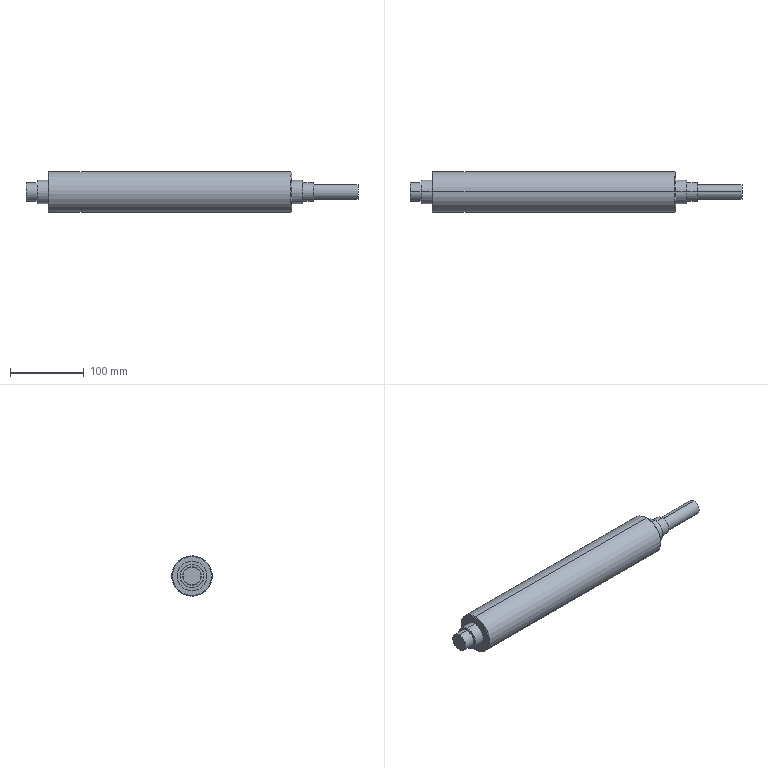Part | SolidWorks | features Chamfer 2, ICE 1, Revolution 1 | 2 solids | 37 faces | box 450 x 55 x 55 mm | volume 841512 mm3 | cylinder 16 | cone 12 | plane 9 | commonest cylinder face diameters 25 x4 32 x4 40 x4 20 x2 55 x2
STEP:
#1=CARTESIAN_POINT('',(390.,0.,-12.));
#2=VERTEX_POINT('',#1);
#3=CARTESIAN_POINT('',(390.,0.,12.));
#4=VERTEX_POINT('',#3);
#5=CARTESIAN_POINT('',(390.,0.,0.));
#6=DIRECTION('',(1.,0.,0.));
#7=DIRECTION('',(0.,0.,1.));
#8=AXIS2_PLACEMENT_3D('',#5,#6,#7);
#9=CIRCLE('',#8,12.);
#10=EDGE_CURVE('',#2,#4,#9,.T.);
#11=ORIENTED_EDGE('',*,*,#10,.F.);
#12=CARTESIAN_POINT('',(389.5,0.,-12.5));
#13=VERTEX_POINT('',#12);
#14=CARTESIAN_POINT('',(389.5,0.,-12.5));
#15=DIRECTION('',(-0.7071,0.,-0.7071));
#16=VECTOR('',#15,1000.);
#17=LINE('',#14,#16);
#18=EDGE_CURVE('',#2,#13,#17,.T.);
#19=ORIENTED_EDGE('',*,*,#18,.T.);
#20=CARTESIAN_POINT('',(389.5,0.,12.5));
#21=VERTEX_POINT('',#20);
#22=CARTESIAN_POINT('',(389.5,0.,0.));
#23=DIRECTION('',(-1.,0.,0.));
#24=DIRECTION('',(0.,0.,1.));
#25=AXIS2_PLACEMENT_3D('',#22,#23,#24);
#26=CIRCLE('',#25,12.5);
#27=EDGE_CURVE('',#21,#13,#26,.T.);
#28=ORIENTED_EDGE('',*,*,#27,.F.);
#29=CARTESIAN_POINT('',(389.5,0.,12.5));
#30=DIRECTION('',(-0.7071,0.,0.7071));
#31=VECTOR('',#30,1000.);
#32=LINE('',#29,#31);
#33=EDGE_CURVE('',#4,#21,#32,.T.);
#34=ORIENTED_EDGE('',*,*,#33,.F.);
#35=EDGE_LOOP('',(#11,#19,#28,#34));
#36=FACE_OUTER_BOUND('',#35,.T.);
#37=CARTESIAN_POINT('',(389.5,0.,0.));
#38=DIRECTION('',(-1.,0.,0.));
#39=DIRECTION('',(0.,0.,1.));
#40=AXIS2_PLACEMENT_3D('',#37,#38,#39);
#41=CONICAL_SURFACE('',#40,12.5,0.7854);
#42=ADVANCED_FACE('',(#36),#41,.T.);
#43=CARTESIAN_POINT('',(375.,0.,-15.5));
#44=VERTEX_POINT('',#43);
#45=CARTESIAN_POINT('',(375.,0.,15.5));
#46=VERTEX_POINT('',#45);
#47=CARTESIAN_POINT('',(375.,0.,0.));
#48=DIRECTION('',(1.,0.,0.));
#49=DIRECTION('',(0.,0.,1.));
#50=AXIS2_PLACEMENT_3D('',#47,#48,#49);
#51=CIRCLE('',#50,15.5);
#52=EDGE_CURVE('',#44,#46,#51,.T.);
#53=ORIENTED_EDGE('',*,*,#52,.F.);
#54=CARTESIAN_POINT('',(374.5,0.,-16.));
#55=VERTEX_POINT('',#54);
#56=CARTESIAN_POINT('',(374.5,0.,-16.));
#57=DIRECTION('',(-0.7071,0.,-0.7071));
#58=VECTOR('',#57,1000.);
#59=LINE('',#56,#58);
#60=EDGE_CURVE('',#44,#55,#59,.T.);
#61=ORIENTED_EDGE('',*,*,#60,.T.);
#62=CARTESIAN_POINT('',(374.5,0.,16.));
#63=VERTEX_POINT('',#62);
#64=CARTESIAN_POINT('',(374.5,0.,0.));
#65=DIRECTION('',(-1.,0.,0.));
#66=DIRECTION('',(0.,0.,1.));
#67=AXIS2_PLACEMENT_3D('',#64,#65,#66);
#68=CIRCLE('',#67,16.);
#69=EDGE_CURVE('',#63,#55,#68,.T.);
#70=ORIENTED_EDGE('',*,*,#69,.F.);
#71=CARTESIAN_POINT('',(374.5,0.,16.));
#72=DIRECTION('',(-0.7071,0.,0.7071));
#73=VECTOR('',#72,1000.);
#74=LINE('',#71,#73);
#75=EDGE_CURVE('',#46,#63,#74,.T.);
#76=ORIENTED_EDGE('',*,*,#75,.F.);
#77=EDGE_LOOP('',(#53,#61,#70,#76));
#78=FACE_OUTER_BOUND('',#77,.T.);
#79=CARTESIAN_POINT('',(374.5,0.,0.));
#80=DIRECTION('',(-1.,0.,0.));
#81=DIRECTION('',(0.,0.,1.));
#82=AXIS2_PLACEMENT_3D('',#79,#80,#81);
#83=CONICAL_SURFACE('',#82,16.,0.7854);
#84=ADVANCED_FACE('',(#78),#83,.T.);
#85=CARTESIAN_POINT('',(15.,0.,15.5));
#86=VERTEX_POINT('',#85);
#87=CARTESIAN_POINT('',(15.,0.,-15.5));
#88=VERTEX_POINT('',#87);
#89=CARTESIAN_POINT('',(15.,0.,0.));
#90=DIRECTION('',(-1.,0.,0.));
#91=DIRECTION('',(0.,0.,-1.));
#92=AXIS2_PLACEMENT_3D('',#89,#90,#91);
#93=CIRCLE('',#92,15.5);
#94=EDGE_CURVE('',#86,#88,#93,.T.);
#95=ORIENTED_EDGE('',*,*,#94,.F.);
#96=CARTESIAN_POINT('',(15.5,0.,16.));
#97=VERTEX_POINT('',#96);
#98=CARTESIAN_POINT('',(15.,0.,15.5));
#99=DIRECTION('',(0.7071,0.,0.7071));
#100=VECTOR('',#99,1000.);
#101=LINE('',#98,#100);
#102=EDGE_CURVE('',#86,#97,#101,.T.);
#103=ORIENTED_EDGE('',*,*,#102,.T.);
#104=CARTESIAN_POINT('',(15.5,0.,-16.));
#105=VERTEX_POINT('',#104);
#106=CARTESIAN_POINT('',(15.5,0.,0.));
#107=DIRECTION('',(1.,0.,0.));
#108=DIRECTION('',(0.,0.,-1.));
#109=AXIS2_PLACEMENT_3D('',#106,#107,#108);
#110=CIRCLE('',#109,16.);
#111=EDGE_CURVE('',#105,#97,#110,.T.);
#112=ORIENTED_EDGE('',*,*,#111,.F.);
#113=CARTESIAN_POINT('',(15.,0.,-15.5));
#114=DIRECTION('',(0.7071,0.,-0.7071));
#115=VECTOR('',#114,1000.);
#116=LINE('',#113,#115);
#117=EDGE_CURVE('',#88,#105,#116,.T.);
#118=ORIENTED_EDGE('',*,*,#117,.F.);
#119=EDGE_LOOP('',(#95,#103,#112,#118));
#120=FACE_OUTER_BOUND('',#119,.T.);
#121=CARTESIAN_POINT('',(15.,0.,0.));
#122=DIRECTION('',(1.,0.,0.));
#123=DIRECTION('',(0.,0.,-1.));
#124=AXIS2_PLACEMENT_3D('',#121,#122,#123);
#125=CONICAL_SURFACE('',#124,15.5,0.7854);
#126=ADVANCED_FACE('',(#120),#125,.T.);
#127=CARTESIAN_POINT('',(0.,0.,12.));
#128=VERTEX_POINT('',#127);
#129=CARTESIAN_POINT('',(0.,0.,-12.));
#130=VERTEX_POINT('',#129);
#131=CARTESIAN_POINT('',(0.,0.,0.));
#132=DIRECTION('',(-1.,0.,0.));
#133=DIRECTION('',(0.,0.,-1.));
#134=AXIS2_PLACEMENT_3D('',#131,#132,#133);
#135=CIRCLE('',#134,12.);
#136=EDGE_CURVE('',#128,#130,#135,.T.);
#137=ORIENTED_EDGE('',*,*,#136,.F.);
#138=CARTESIAN_POINT('',(0.5,0.,12.5));
#139=VERTEX_POINT('',#138);
#140=CARTESIAN_POINT('',(0.,0.,12.));
#141=DIRECTION('',(0.7071,0.,0.7071));
#142=VECTOR('',#141,1000.);
#143=LINE('',#140,#142);
#144=EDGE_CURVE('',#128,#139,#143,.T.);
#145=ORIENTED_EDGE('',*,*,#144,.T.);
#146=CARTESIAN_POINT('',(0.5,0.,-12.5));
#147=VERTEX_POINT('',#146);
#148=CARTESIAN_POINT('',(0.5,0.,0.));
#149=DIRECTION('',(1.,0.,0.));
#150=DIRECTION('',(0.,0.,-1.));
#151=AXIS2_PLACEMENT_3D('',#148,#149,#150);
#152=CIRCLE('',#151,12.5);
#153=EDGE_CURVE('',#147,#139,#152,.T.);
#154=ORIENTED_EDGE('',*,*,#153,.F.);
#155=CARTESIAN_POINT('',(0.,0.,-12.));
#156=DIRECTION('',(0.7071,0.,-0.7071));
#157=VECTOR('',#156,1000.);
#158=LINE('',#155,#157);
#159=EDGE_CURVE('',#130,#147,#158,.T.);
#160=ORIENTED_EDGE('',*,*,#159,.F.);
#161=EDGE_LOOP('',(#137,#145,#154,#160));
#162=FACE_OUTER_BOUND('',#161,.T.);
#163=CARTESIAN_POINT('',(0.,0.,0.));
#164=DIRECTION('',(1.,0.,0.));
#165=DIRECTION('',(0.,0.,-1.));
#166=AXIS2_PLACEMENT_3D('',#163,#164,#165);
#167=CONICAL_SURFACE('',#166,12.,0.7854);
#168=ADVANCED_FACE('',(#162),#167,.T.);
#169=CARTESIAN_POINT('',(15.,0.,12.5));
#170=VERTEX_POINT('',#169);
#171=CARTESIAN_POINT('',(15.,0.,-12.5));
#172=VERTEX_POINT('',#171);
#173=CARTESIAN_POINT('',(15.,0.,0.));
#174=DIRECTION('',(-1.,0.,0.));
#175=DIRECTION('',(0.,0.,1.));
#176=AXIS2_PLACEMENT_3D('',#173,#174,#175);
#177=CIRCLE('',#176,12.5);
#178=EDGE_CURVE('',#170,#172,#177,.T.);
#179=ORIENTED_EDGE('',*,*,#178,.T.);
#180=CARTESIAN_POINT('',(0.,0.,-12.5));
#181=DIRECTION('',(-1.,0.,0.));
#182=VECTOR('',#181,1000.);
#183=LINE('',#180,#182);
#184=EDGE_CURVE('',#172,#147,#183,.T.);
#185=ORIENTED_EDGE('',*,*,#184,.T.);
#186=ORIENTED_EDGE('',*,*,#153,.T.);
#187=CARTESIAN_POINT('',(0.,0.,12.5));
#188=DIRECTION('',(-1.,0.,0.));
#189=VECTOR('',#188,1000.);
#190=LINE('',#187,#189);
#191=EDGE_CURVE('',#170,#139,#190,.T.);
#192=ORIENTED_EDGE('',*,*,#191,.F.);
#193=EDGE_LOOP('',(#179,#185,#186,#192));
#194=FACE_OUTER_BOUND('',#193,.T.);
#195=CARTESIAN_POINT('',(0.,0.,0.));
#196=DIRECTION('',(-1.,0.,0.));
#197=DIRECTION('',(0.,0.,1.));
#198=AXIS2_PLACEMENT_3D('',#195,#196,#197);
#199=CYLINDRICAL_SURFACE('',#198,12.5);
#200=ADVANCED_FACE('',(#194),#199,.T.);
#201=CARTESIAN_POINT('',(30.,0.,16.));
#202=VERTEX_POINT('',#201);
#203=CARTESIAN_POINT('',(30.,0.,-16.));
#204=VERTEX_POINT('',#203);
#205=CARTESIAN_POINT('',(30.,0.,0.));
#206=DIRECTION('',(-1.,0.,0.));
#207=DIRECTION('',(0.,0.,1.));
#208=AXIS2_PLACEMENT_3D('',#205,#206,#207);
#209=CIRCLE('',#208,16.);
#210=EDGE_CURVE('',#202,#204,#209,.T.);
#211=ORIENTED_EDGE('',*,*,#210,.T.);
#212=CARTESIAN_POINT('',(0.,0.,-16.));
#213=DIRECTION('',(-1.,0.,0.));
#214=VECTOR('',#213,1000.);
#215=LINE('',#212,#214);
#216=EDGE_CURVE('',#204,#105,#215,.T.);
#217=ORIENTED_EDGE('',*,*,#216,.T.);
#218=ORIENTED_EDGE('',*,*,#111,.T.);
#219=CARTESIAN_POINT('',(0.,0.,16.));
#220=DIRECTION('',(-1.,0.,0.));
#221=VECTOR('',#220,1000.);
#222=LINE('',#219,#221);
#223=EDGE_CURVE('',#202,#97,#222,.T.);
#224=ORIENTED_EDGE('',*,*,#223,.F.);
#225=EDGE_LOOP('',(#211,#217,#218,#224));
#226=FACE_OUTER_BOUND('',#225,.T.);
#227=CARTESIAN_POINT('',(0.,0.,0.));
#228=DIRECTION('',(-1.,0.,0.));
#229=DIRECTION('',(0.,0.,1.));
#230=AXIS2_PLACEMENT_3D('',#227,#228,#229);
#231=CYLINDRICAL_SURFACE('',#230,16.);
#232=ADVANCED_FACE('',(#226),#231,.T.);
#233=CARTESIAN_POINT('',(360.,0.,20.));
#234=VERTEX_POINT('',#233);
#235=CARTESIAN_POINT('',(360.,0.,-20.));
#236=VERTEX_POINT('',#235);
#237=CARTESIAN_POINT('',(360.,0.,0.));
#238=DIRECTION('',(-1.,0.,0.));
#239=DIRECTION('',(0.,0.,1.));
#240=AXIS2_PLACEMENT_3D('',#237,#238,#239);
#241=CIRCLE('',#240,20.);
#242=EDGE_CURVE('',#234,#236,#241,.T.);
#243=ORIENTED_EDGE('',*,*,#242,.T.);
#244=CARTESIAN_POINT('',(30.,0.,-20.));
#245=VERTEX_POINT('',#244);
#246=CARTESIAN_POINT('',(0.,0.,-20.));
#247=DIRECTION('',(-1.,0.,0.));
#248=VECTOR('',#247,1000.);
#249=LINE('',#246,#248);
#250=EDGE_CURVE('',#236,#245,#249,.T.);
#251=ORIENTED_EDGE('',*,*,#250,.T.);
#252=CARTESIAN_POINT('',(30.,0.,20.));
#253=VERTEX_POINT('',#252);
#254=CARTESIAN_POINT('',(30.,0.,0.));
#255=DIRECTION('',(-1.,0.,0.));
#256=DIRECTION('',(0.,0.,1.));
#257=AXIS2_PLACEMENT_3D('',#254,#255,#256);
#258=CIRCLE('',#257,20.);
#259=EDGE_CURVE('',#253,#245,#258,.T.);
#260=ORIENTED_EDGE('',*,*,#259,.F.);
#261=CARTESIAN_POINT('',(0.,0.,20.));
#262=DIRECTION('',(-1.,0.,0.));
#263=VECTOR('',#262,1000.);
#264=LINE('',#261,#263);
#265=EDGE_CURVE('',#234,#253,#264,.T.);
#266=ORIENTED_EDGE('',*,*,#265,.F.);
#267=EDGE_LOOP('',(#243,#251,#260,#266));
#268=FACE_OUTER_BOUND('',#267,.T.);
#269=CARTESIAN_POINT('',(0.,0.,0.));
#270=DIRECTION('',(-1.,0.,0.));
#271=DIRECTION('',(0.,0.,1.));
#272=AXIS2_PLACEMENT_3D('',#269,#270,#271);
#273=CYLINDRICAL_SURFACE('',#272,20.);
#274=ADVANCED_FACE('',(#268),#273,.T.);
#275=ORIENTED_EDGE('',*,*,#69,.T.);
#276=CARTESIAN_POINT('',(360.,0.,-16.));
#277=VERTEX_POINT('',#276);
#278=CARTESIAN_POINT('',(0.,0.,-16.));
#279=DIRECTION('',(-1.,0.,0.));
#280=VECTOR('',#279,1000.);
#281=LINE('',#278,#280);
#282=EDGE_CURVE('',#55,#277,#281,.T.);
#283=ORIENTED_EDGE('',*,*,#282,.T.);
#284=CARTESIAN_POINT('',(360.,0.,16.));
#285=VERTEX_POINT('',#284);
#286=CARTESIAN_POINT('',(360.,0.,0.));
#287=DIRECTION('',(-1.,0.,0.));
#288=DIRECTION('',(0.,0.,1.));
#289=AXIS2_PLACEMENT_3D('',#286,#287,#288);
#290=CIRCLE('',#289,16.);
#291=EDGE_CURVE('',#285,#277,#290,.T.);
#292=ORIENTED_EDGE('',*,*,#291,.F.);
#293=CARTESIAN_POINT('',(0.,0.,16.));
#294=DIRECTION('',(-1.,0.,0.));
#295=VECTOR('',#294,1000.);
#296=LINE('',#293,#295);
#297=EDGE_CURVE('',#63,#285,#296,.T.);
#298=ORIENTED_EDGE('',*,*,#297,.F.);
#299=EDGE_LOOP('',(#275,#283,#292,#298));
#300=FACE_OUTER_BOUND('',#299,.T.);
#301=CARTESIAN_POINT('',(0.,0.,0.));
#302=DIRECTION('',(-1.,0.,0.));
#303=DIRECTION('',(0.,0.,1.));
#304=AXIS2_PLACEMENT_3D('',#301,#302,#303);
#305=CYLINDRICAL_SURFACE('',#304,16.);
#306=ADVANCED_FACE('',(#300),#305,.T.);
#307=ORIENTED_EDGE('',*,*,#27,.T.);
#308=CARTESIAN_POINT('',(375.,0.,-12.5));
#309=VERTEX_POINT('',#308);
#310=CARTESIAN_POINT('',(0.,0.,-12.5));
#311=DIRECTION('',(-1.,0.,0.));
#312=VECTOR('',#311,1000.);
#313=LINE('',#310,#312);
#314=EDGE_CURVE('',#13,#309,#313,.T.);
#315=ORIENTED_EDGE('',*,*,#314,.T.);
#316=CARTESIAN_POINT('',(375.,0.,12.5));
#317=VERTEX_POINT('',#316);
#318=CARTESIAN_POINT('',(375.,0.,0.));
#319=DIRECTION('',(-1.,0.,0.));
#320=DIRECTION('',(0.,0.,1.));
#321=AXIS2_PLACEMENT_3D('',#318,#319,#320);
#322=CIRCLE('',#321,12.5);
#323=EDGE_CURVE('',#317,#309,#322,.T.);
#324=ORIENTED_EDGE('',*,*,#323,.F.);
#325=CARTESIAN_POINT('',(0.,0.,12.5));
#326=DIRECTION('',(-1.,0.,0.));
#327=VECTOR('',#326,1000.);
#328=LINE('',#325,#327);
#329=EDGE_CURVE('',#21,#317,#328,.T.);
#330=ORIENTED_EDGE('',*,*,#329,.F.);
#331=EDGE_LOOP('',(#307,#315,#324,#330));
#332=FACE_OUTER_BOUND('',#331,.T.);
#333=CARTESIAN_POINT('',(0.,0.,0.));
#334=DIRECTION('',(-1.,0.,0.));
#335=DIRECTION('',(0.,0.,1.));
#336=AXIS2_PLACEMENT_3D('',#333,#334,#335);
#337=CYLINDRICAL_SURFACE('',#336,12.5);
#338=ADVANCED_FACE('',(#332),#337,.T.);
#339=CARTESIAN_POINT('',(450.,0.,10.));
#340=VERTEX_POINT('',#339);
#341=CARTESIAN_POINT('',(450.,0.,-10.));
#342=VERTEX_POINT('',#341);
#343=CARTESIAN_POINT('',(450.,0.,0.));
#344=DIRECTION('',(-1.,0.,0.));
#345=DIRECTION('',(0.,0.,1.));
#346=AXIS2_PLACEMENT_3D('',#343,#344,#345);
#347=CIRCLE('',#346,10.);
#348=EDGE_CURVE('',#340,#342,#347,.T.);
#349=ORIENTED_EDGE('',*,*,#348,.T.);
#350=CARTESIAN_POINT('',(390.,0.,-10.));
#351=VERTEX_POINT('',#350);
#352=CARTESIAN_POINT('',(0.,0.,-10.));
#353=DIRECTION('',(-1.,0.,0.));
#354=VECTOR('',#353,1000.);
#355=LINE('',#352,#354);
#356=EDGE_CURVE('',#342,#351,#355,.T.);
#357=ORIENTED_EDGE('',*,*,#356,.T.);
#358=CARTESIAN_POINT('',(390.,0.,10.));
#359=VERTEX_POINT('',#358);
#360=CARTESIAN_POINT('',(390.,0.,0.));
#361=DIRECTION('',(-1.,0.,0.));
#362=DIRECTION('',(0.,0.,1.));
#363=AXIS2_PLACEMENT_3D('',#360,#361,#362);
#364=CIRCLE('',#363,10.);
#365=EDGE_CURVE('',#359,#351,#364,.T.);
#366=ORIENTED_EDGE('',*,*,#365,.F.);
#367=CARTESIAN_POINT('',(0.,0.,10.));
#368=DIRECTION('',(-1.,0.,0.));
#369=VECTOR('',#368,1000.);
#370=LINE('',#367,#369);
#371=EDGE_CURVE('',#340,#359,#370,.T.);
#372=ORIENTED_EDGE('',*,*,#371,.F.);
#373=EDGE_LOOP('',(#349,#357,#366,#372));
#374=FACE_OUTER_BOUND('',#373,.T.);
#375=CARTESIAN_POINT('',(0.,0.,0.));
#376=DIRECTION('',(-1.,0.,0.));
#377=DIRECTION('',(0.,0.,1.));
#378=AXIS2_PLACEMENT_3D('',#375,#376,#377);
#379=CYLINDRICAL_SURFACE('',#378,10.);
#380=ADVANCED_FACE('',(#374),#379,.T.);
#381=ORIENTED_EDGE('',*,*,#348,.F.);
#382=CARTESIAN_POINT('',(450.,0.,0.));
#383=DIRECTION('',(-1.,0.,0.));
#384=DIRECTION('',(0.,0.,1.));
#385=AXIS2_PLACEMENT_3D('',#382,#383,#384);
#386=CIRCLE('',#385,10.);
#387=EDGE_CURVE('',#342,#340,#386,.T.);
#388=ORIENTED_EDGE('',*,*,#387,.F.);
#389=EDGE_LOOP('',(#381,#388));
#390=FACE_OUTER_BOUND('',#389,.T.);
#391=CARTESIAN_POINT('',(450.,0.,0.));
#392=DIRECTION('',(-1.,0.,0.));
#393=DIRECTION('',(0.,0.,1.));
#394=AXIS2_PLACEMENT_3D('',#391,#392,#393);
#395=PLANE('',#394);
#396=ADVANCED_FACE('',(#390),#395,.F.);
#397=ORIENTED_EDGE('',*,*,#356,.F.);
#398=ORIENTED_EDGE('',*,*,#387,.T.);
#399=ORIENTED_EDGE('',*,*,#371,.T.);
#400=CARTESIAN_POINT('',(390.,0.,0.));
#401=DIRECTION('',(-1.,0.,0.));
#402=DIRECTION('',(0.,0.,1.));
#403=AXIS2_PLACEMENT_3D('',#400,#401,#402);
#404=CIRCLE('',#403,10.);
#405=EDGE_CURVE('',#351,#359,#404,.T.);
#406=ORIENTED_EDGE('',*,*,#405,.F.);
#407=EDGE_LOOP('',(#397,#398,#399,#406));
#408=FACE_OUTER_BOUND('',#407,.T.);
#409=CARTESIAN_POINT('',(0.,0.,0.));
#410=DIRECTION('',(-1.,0.,0.));
#411=DIRECTION('',(0.,0.,1.));
#412=AXIS2_PLACEMENT_3D('',#409,#410,#411);
#413=CYLINDRICAL_SURFACE('',#412,10.);
#414=ADVANCED_FACE('',(#408),#413,.T.);
#415=CARTESIAN_POINT('',(390.,0.,0.));
#416=DIRECTION('',(1.,0.,0.));
#417=DIRECTION('',(0.,0.,1.));
#418=AXIS2_PLACEMENT_3D('',#415,#416,#417);
#419=CIRCLE('',#418,12.);
#420=EDGE_CURVE('',#4,#2,#419,.T.);
#421=ORIENTED_EDGE('',*,*,#420,.T.);
#422=ORIENTED_EDGE('',*,*,#10,.T.);
#423=EDGE_LOOP('',(#421,#422));
#424=FACE_OUTER_BOUND('',#423,.T.);
#425=ORIENTED_EDGE('',*,*,#365,.T.);
#426=ORIENTED_EDGE('',*,*,#405,.T.);
#427=EDGE_LOOP('',(#425,#426));
#428=FACE_BOUND('',#427,.T.);
#429=CARTESIAN_POINT('',(390.,10.,0.));
#430=DIRECTION('',(-1.,0.,0.));
#431=DIRECTION('',(0.,0.,1.));
#432=AXIS2_PLACEMENT_3D('',#429,#430,#431);
#433=PLANE('',#432);
#434=ADVANCED_FACE('',(#424,#428),#433,.F.);
#435=ORIENTED_EDGE('',*,*,#314,.F.);
#436=CARTESIAN_POINT('',(389.5,0.,0.));
#437=DIRECTION('',(-1.,0.,0.));
#438=DIRECTION('',(0.,0.,1.));
#439=AXIS2_PLACEMENT_3D('',#436,#437,#438);
#440=CIRCLE('',#439,12.5);
#441=EDGE_CURVE('',#13,#21,#440,.T.);
#442=ORIENTED_EDGE('',*,*,#441,.T.);
#443=ORIENTED_EDGE('',*,*,#329,.T.);
#444=CARTESIAN_POINT('',(375.,0.,0.));
#445=DIRECTION('',(-1.,0.,0.));
#446=DIRECTION('',(0.,0.,1.));
#447=AXIS2_PLACEMENT_3D('',#444,#445,#446);
#448=CIRCLE('',#447,12.5);
#449=EDGE_CURVE('',#309,#317,#448,.T.);
#450=ORIENTED_EDGE('',*,*,#449,.F.);
#451=EDGE_LOOP('',(#435,#442,#443,#450));
#452=FACE_OUTER_BOUND('',#451,.T.);
#453=CARTESIAN_POINT('',(0.,0.,0.));
#454=DIRECTION('',(-1.,0.,0.));
#455=DIRECTION('',(0.,0.,1.));
#456=AXIS2_PLACEMENT_3D('',#453,#454,#455);
#457=CYLINDRICAL_SURFACE('',#456,12.5);
#458=ADVANCED_FACE('',(#452),#457,.T.);
#459=CARTESIAN_POINT('',(375.,0.,0.));
#460=DIRECTION('',(1.,0.,0.));
#461=DIRECTION('',(0.,0.,1.));
#462=AXIS2_PLACEMENT_3D('',#459,#460,#461);
#463=CIRCLE('',#462,15.5);
#464=EDGE_CURVE('',#46,#44,#463,.T.);
#465=ORIENTED_EDGE('',*,*,#464,.T.);
#466=ORIENTED_EDGE('',*,*,#52,.T.);
#467=EDGE_LOOP('',(#465,#466));
#468=FACE_OUTER_BOUND('',#467,.T.);
#469=ORIENTED_EDGE('',*,*,#323,.T.);
#470=ORIENTED_EDGE('',*,*,#449,.T.);
#471=EDGE_LOOP('',(#469,#470));
#472=FACE_BOUND('',#471,.T.);
#473=CARTESIAN_POINT('',(375.,12.5,0.));
#474=DIRECTION('',(-1.,0.,0.));
#475=DIRECTION('',(0.,0.,1.));
#476=AXIS2_PLACEMENT_3D('',#473,#474,#475);
#477=PLANE('',#476);
#478=ADVANCED_FACE('',(#468,#472),#477,.F.);
#479=ORIENTED_EDGE('',*,*,#282,.F.);
#480=CARTESIAN_POINT('',(374.5,0.,0.));
#481=DIRECTION('',(-1.,0.,0.));
#482=DIRECTION('',(0.,0.,1.));
#483=AXIS2_PLACEMENT_3D('',#480,#481,#482);
#484=CIRCLE('',#483,16.);
#485=EDGE_CURVE('',#55,#63,#484,.T.);
#486=ORIENTED_EDGE('',*,*,#485,.T.);
#487=ORIENTED_EDGE('',*,*,#297,.T.);
#488=CARTESIAN_POINT('',(360.,0.,0.));
#489=DIRECTION('',(-1.,0.,0.));
#490=DIRECTION('',(0.,0.,1.));
#491=AXIS2_PLACEMENT_3D('',#488,#489,#490);
#492=CIRCLE('',#491,16.);
#493=EDGE_CURVE('',#277,#285,#492,.T.);
#494=ORIENTED_EDGE('',*,*,#493,.F.);
#495=EDGE_LOOP('',(#479,#486,#487,#494));
#496=FACE_OUTER_BOUND('',#495,.T.);
#497=CARTESIAN_POINT('',(0.,0.,0.));
#498=DIRECTION('',(-1.,0.,0.));
#499=DIRECTION('',(0.,0.,1.));
#500=AXIS2_PLACEMENT_3D('',#497,#498,#499);
#501=CYLINDRICAL_SURFACE('',#500,16.);
#502=ADVANCED_FACE('',(#496),#501,.T.);
#503=ORIENTED_EDGE('',*,*,#242,.F.);
#504=CARTESIAN_POINT('',(360.,0.,0.));
#505=DIRECTION('',(-1.,0.,0.));
#506=DIRECTION('',(0.,0.,1.));
#507=AXIS2_PLACEMENT_3D('',#504,#505,#506);
#508=CIRCLE('',#507,20.);
#509=EDGE_CURVE('',#236,#234,#508,.T.);
#510=ORIENTED_EDGE('',*,*,#509,.F.);
#511=EDGE_LOOP('',(#503,#510));
#512=FACE_OUTER_BOUND('',#511,.T.);
#513=ORIENTED_EDGE('',*,*,#291,.T.);
#514=ORIENTED_EDGE('',*,*,#493,.T.);
#515=EDGE_LOOP('',(#513,#514));
#516=FACE_BOUND('',#515,.T.);
#517=CARTESIAN_POINT('',(360.,16.,0.));
#518=DIRECTION('',(-1.,0.,0.));
#519=DIRECTION('',(0.,0.,1.));
#520=AXIS2_PLACEMENT_3D('',#517,#518,#519);
#521=PLANE('',#520);
#522=ADVANCED_FACE('',(#512,#516),#521,.F.);
#523=ORIENTED_EDGE('',*,*,#250,.F.);
#524=ORIENTED_EDGE('',*,*,#509,.T.);
#525=ORIENTED_EDGE('',*,*,#265,.T.);
#526=CARTESIAN_POINT('',(30.,0.,0.));
#527=DIRECTION('',(-1.,0.,0.));
#528=DIRECTION('',(0.,0.,1.));
#529=AXIS2_PLACEMENT_3D('',#526,#527,#528);
#530=CIRCLE('',#529,20.);
#531=EDGE_CURVE('',#245,#253,#530,.T.);
#532=ORIENTED_EDGE('',*,*,#531,.F.);
#533=EDGE_LOOP('',(#523,#524,#525,#532));
#534=FACE_OUTER_BOUND('',#533,.T.);
#535=CARTESIAN_POINT('',(0.,0.,0.));
#536=DIRECTION('',(-1.,0.,0.));
#537=DIRECTION('',(0.,0.,1.));
#538=AXIS2_PLACEMENT_3D('',#535,#536,#537);
#539=CYLINDRICAL_SURFACE('',#538,20.);
#540=ADVANCED_FACE('',(#534),#539,.T.);
#541=ORIENTED_EDGE('',*,*,#210,.F.);
#542=CARTESIAN_POINT('',(30.,0.,0.));
#543=DIRECTION('',(-1.,0.,0.));
#544=DIRECTION('',(0.,0.,1.));
#545=AXIS2_PLACEMENT_3D('',#542,#543,#544);
#546=CIRCLE('',#545,16.);
#547=EDGE_CURVE('',#204,#202,#546,.T.);
#548=ORIENTED_EDGE('',*,*,#547,.F.);
#549=EDGE_LOOP('',(#541,#548));
#550=FACE_BOUND('',#549,.T.);
#551=ORIENTED_EDGE('',*,*,#259,.T.);
#552=ORIENTED_EDGE('',*,*,#531,.T.);
#553=EDGE_LOOP('',(#551,#552));
#554=FACE_OUTER_BOUND('',#553,.T.);
#555=CARTESIAN_POINT('',(30.,16.,0.));
#556=DIRECTION('',(1.,0.,0.));
#557=DIRECTION('',(0.,0.,-1.));
#558=AXIS2_PLACEMENT_3D('',#555,#556,#557);
#559=PLANE('',#558);
#560=ADVANCED_FACE('',(#550,#554),#559,.F.);
#561=ORIENTED_EDGE('',*,*,#216,.F.);
#562=ORIENTED_EDGE('',*,*,#547,.T.);
#563=ORIENTED_EDGE('',*,*,#223,.T.);
#564=CARTESIAN_POINT('',(15.5,0.,0.));
#565=DIRECTION('',(1.,0.,0.));
#566=DIRECTION('',(0.,0.,-1.));
#567=AXIS2_PLACEMENT_3D('',#564,#565,#566);
#568=CIRCLE('',#567,16.);
#569=EDGE_CURVE('',#97,#105,#568,.T.);
#570=ORIENTED_EDGE('',*,*,#569,.T.);
#571=EDGE_LOOP('',(#561,#562,#563,#570));
#572=FACE_OUTER_BOUND('',#571,.T.);
#573=CARTESIAN_POINT('',(0.,0.,0.));
#574=DIRECTION('',(-1.,0.,0.));
#575=DIRECTION('',(0.,0.,1.));
#576=AXIS2_PLACEMENT_3D('',#573,#574,#575);
#577=CYLINDRICAL_SURFACE('',#576,16.);
#578=ADVANCED_FACE('',(#572),#577,.T.);
#579=CARTESIAN_POINT('',(15.,0.,0.));
#580=DIRECTION('',(-1.,0.,0.));
#581=DIRECTION('',(0.,0.,-1.));
#582=AXIS2_PLACEMENT_3D('',#579,#580,#581);
#583=CIRCLE('',#582,15.5);
#584=EDGE_CURVE('',#88,#86,#583,.T.);
#585=ORIENTED_EDGE('',*,*,#584,.T.);
#586=ORIENTED_EDGE('',*,*,#94,.T.);
#587=EDGE_LOOP('',(#585,#586));
#588=FACE_OUTER_BOUND('',#587,.T.);
#589=ORIENTED_EDGE('',*,*,#178,.F.);
#590=CARTESIAN_POINT('',(15.,0.,0.));
#591=DIRECTION('',(-1.,0.,0.));
#592=DIRECTION('',(0.,0.,1.));
#593=AXIS2_PLACEMENT_3D('',#590,#591,#592);
#594=CIRCLE('',#593,12.5);
#595=EDGE_CURVE('',#172,#170,#594,.T.);
#596=ORIENTED_EDGE('',*,*,#595,.F.);
#597=EDGE_LOOP('',(#589,#596));
#598=FACE_BOUND('',#597,.T.);
#599=CARTESIAN_POINT('',(15.,12.5,0.));
#600=DIRECTION('',(1.,0.,0.));
#601=DIRECTION('',(0.,0.,-1.));
#602=AXIS2_PLACEMENT_3D('',#599,#600,#601);
#603=PLANE('',#602);
#604=ADVANCED_FACE('',(#588,#598),#603,.F.);
#605=ORIENTED_EDGE('',*,*,#184,.F.);
#606=ORIENTED_EDGE('',*,*,#595,.T.);
#607=ORIENTED_EDGE('',*,*,#191,.T.);
#608=CARTESIAN_POINT('',(0.5,0.,0.));
#609=DIRECTION('',(1.,0.,0.));
#610=DIRECTION('',(0.,0.,-1.));
#611=AXIS2_PLACEMENT_3D('',#608,#609,#610);
#612=CIRCLE('',#611,12.5);
#613=EDGE_CURVE('',#139,#147,#612,.T.);
#614=ORIENTED_EDGE('',*,*,#613,.T.);
#615=EDGE_LOOP('',(#605,#606,#607,#614));
#616=FACE_OUTER_BOUND('',#615,.T.);
#617=CARTESIAN_POINT('',(0.,0.,0.));
#618=DIRECTION('',(-1.,0.,0.));
#619=DIRECTION('',(0.,0.,1.));
#620=AXIS2_PLACEMENT_3D('',#617,#618,#619);
#621=CYLINDRICAL_SURFACE('',#620,12.5);
#622=ADVANCED_FACE('',(#616),#621,.T.);
#623=CARTESIAN_POINT('',(0.,0.,0.));
#624=DIRECTION('',(-1.,0.,0.));
#625=DIRECTION('',(0.,0.,-1.));
#626=AXIS2_PLACEMENT_3D('',#623,#624,#625);
#627=CIRCLE('',#626,12.);
#628=EDGE_CURVE('',#130,#128,#627,.T.);
#629=ORIENTED_EDGE('',*,*,#628,.T.);
#630=ORIENTED_EDGE('',*,*,#136,.T.);
#631=EDGE_LOOP('',(#629,#630));
#632=FACE_OUTER_BOUND('',#631,.T.);
#633=CARTESIAN_POINT('',(0.,0.,0.));
#634=DIRECTION('',(1.,0.,0.));
#635=DIRECTION('',(0.,0.,-1.));
#636=AXIS2_PLACEMENT_3D('',#633,#634,#635);
#637=PLANE('',#636);
#638=ADVANCED_FACE('',(#632),#637,.F.);
#639=ORIENTED_EDGE('',*,*,#144,.F.);
#640=ORIENTED_EDGE('',*,*,#628,.F.);
#641=ORIENTED_EDGE('',*,*,#159,.T.);
#642=ORIENTED_EDGE('',*,*,#613,.F.);
#643=EDGE_LOOP('',(#639,#640,#641,#642));
#644=FACE_OUTER_BOUND('',#643,.T.);
#645=CARTESIAN_POINT('',(0.,0.,0.));
#646=DIRECTION('',(1.,0.,0.));
#647=DIRECTION('',(0.,0.,-1.));
#648=AXIS2_PLACEMENT_3D('',#645,#646,#647);
#649=CONICAL_SURFACE('',#648,12.,0.7854);
#650=ADVANCED_FACE('',(#644),#649,.T.);
#651=ORIENTED_EDGE('',*,*,#102,.F.);
#652=ORIENTED_EDGE('',*,*,#584,.F.);
#653=ORIENTED_EDGE('',*,*,#117,.T.);
#654=ORIENTED_EDGE('',*,*,#569,.F.);
#655=EDGE_LOOP('',(#651,#652,#653,#654));
#656=FACE_OUTER_BOUND('',#655,.T.);
#657=CARTESIAN_POINT('',(15.,0.,0.));
#658=DIRECTION('',(1.,0.,0.));
#659=DIRECTION('',(0.,0.,-1.));
#660=AXIS2_PLACEMENT_3D('',#657,#658,#659);
#661=CONICAL_SURFACE('',#660,15.5,0.7854);
#662=ADVANCED_FACE('',(#656),#661,.T.);
#663=ORIENTED_EDGE('',*,*,#60,.F.);
#664=ORIENTED_EDGE('',*,*,#464,.F.);
#665=ORIENTED_EDGE('',*,*,#75,.T.);
#666=ORIENTED_EDGE('',*,*,#485,.F.);
#667=EDGE_LOOP('',(#663,#664,#665,#666));
#668=FACE_OUTER_BOUND('',#667,.T.);
#669=CARTESIAN_POINT('',(374.5,0.,0.));
#670=DIRECTION('',(-1.,0.,0.));
#671=DIRECTION('',(0.,0.,1.));
#672=AXIS2_PLACEMENT_3D('',#669,#670,#671);
#673=CONICAL_SURFACE('',#672,16.,0.7854);
#674=ADVANCED_FACE('',(#668),#673,.T.);
#675=ORIENTED_EDGE('',*,*,#18,.F.);
#676=ORIENTED_EDGE('',*,*,#420,.F.);
#677=ORIENTED_EDGE('',*,*,#33,.T.);
#678=ORIENTED_EDGE('',*,*,#441,.F.);
#679=EDGE_LOOP('',(#675,#676,#677,#678));
#680=FACE_OUTER_BOUND('',#679,.T.);
#681=CARTESIAN_POINT('',(389.5,0.,0.));
#682=DIRECTION('',(-1.,0.,0.));
#683=DIRECTION('',(0.,0.,1.));
#684=AXIS2_PLACEMENT_3D('',#681,#682,#683);
#685=CONICAL_SURFACE('',#684,12.5,0.7854);
#686=ADVANCED_FACE('',(#680),#685,.T.);
#687=CLOSED_SHELL('',(#42,#84,#126,#168,#200,#232,#274,#306,#338,#380,#396,#414,#434,#458,#478,#502,#522,#540,#560,#578,#604,#622,#638,#650,#662,#674,#686));
#688=MANIFOLD_SOLID_BREP('',#687);
#689=CARTESIAN_POINT('',(30.,0.,26.5));
#690=VERTEX_POINT('',#689);
#691=CARTESIAN_POINT('',(30.,0.,-26.5));
#692=VERTEX_POINT('',#691);
#693=CARTESIAN_POINT('',(30.,0.,0.));
#694=DIRECTION('',(-1.,0.,0.));
#695=DIRECTION('',(0.,0.,-1.));
#696=AXIS2_PLACEMENT_3D('',#693,#694,#695);
#697=CIRCLE('',#696,26.5);
#698=EDGE_CURVE('',#690,#692,#697,.T.);
#699=ORIENTED_EDGE('',*,*,#698,.F.);
#700=CARTESIAN_POINT('',(31.,0.,27.5));
#701=VERTEX_POINT('',#700);
#702=CARTESIAN_POINT('',(30.,0.,26.5));
#703=DIRECTION('',(0.7071,0.,0.7071));
#704=VECTOR('',#703,1000.);
#705=LINE('',#702,#704);
#706=EDGE_CURVE('',#690,#701,#705,.T.);
#707=ORIENTED_EDGE('',*,*,#706,.T.);
#708=CARTESIAN_POINT('',(31.,0.,-27.5));
#709=VERTEX_POINT('',#708);
#710=CARTESIAN_POINT('',(31.,0.,0.));
#711=DIRECTION('',(1.,0.,0.));
#712=DIRECTION('',(0.,0.,-1.));
#713=AXIS2_PLACEMENT_3D('',#710,#711,#712);
#714=CIRCLE('',#713,27.5);
#715=EDGE_CURVE('',#709,#701,#714,.T.);
#716=ORIENTED_EDGE('',*,*,#715,.F.);
#717=CARTESIAN_POINT('',(30.,0.,-26.5));
#718=DIRECTION('',(0.7071,0.,-0.7071));
#719=VECTOR('',#718,1000.);
#720=LINE('',#717,#719);
#721=EDGE_CURVE('',#692,#709,#720,.T.);
#722=ORIENTED_EDGE('',*,*,#721,.F.);
#723=EDGE_LOOP('',(#699,#707,#716,#722));
#724=FACE_OUTER_BOUND('',#723,.T.);
#725=CARTESIAN_POINT('',(30.,0.,0.));
#726=DIRECTION('',(1.,0.,0.));
#727=DIRECTION('',(0.,0.,-1.));
#728=AXIS2_PLACEMENT_3D('',#725,#726,#727);
#729=CONICAL_SURFACE('',#728,26.5,0.7854);
#730=ADVANCED_FACE('',(#724),#729,.T.);
#731=CARTESIAN_POINT('',(360.,0.,-26.5));
#732=VERTEX_POINT('',#731);
#733=CARTESIAN_POINT('',(360.,0.,26.5));
#734=VERTEX_POINT('',#733);
#735=CARTESIAN_POINT('',(360.,0.,0.));
#736=DIRECTION('',(1.,0.,0.));
#737=DIRECTION('',(0.,0.,-1.));
#738=AXIS2_PLACEMENT_3D('',#735,#736,#737);
#739=CIRCLE('',#738,26.5);
#740=EDGE_CURVE('',#732,#734,#739,.T.);
#741=ORIENTED_EDGE('',*,*,#740,.F.);
#742=CARTESIAN_POINT('',(359.,0.,-27.5));
#743=VERTEX_POINT('',#742);
#744=CARTESIAN_POINT('',(360.,0.,-26.5));
#745=DIRECTION('',(-0.7071,0.,-0.7071));
#746=VECTOR('',#745,1000.);
#747=LINE('',#744,#746);
#748=EDGE_CURVE('',#732,#743,#747,.T.);
#749=ORIENTED_EDGE('',*,*,#748,.T.);
#750=CARTESIAN_POINT('',(359.,0.,27.5));
#751=VERTEX_POINT('',#750);
#752=CARTESIAN_POINT('',(359.,0.,0.));
#753=DIRECTION('',(-1.,0.,0.));
#754=DIRECTION('',(0.,0.,-1.));
#755=AXIS2_PLACEMENT_3D('',#752,#753,#754);
#756=CIRCLE('',#755,27.5);
#757=EDGE_CURVE('',#751,#743,#756,.T.);
#758=ORIENTED_EDGE('',*,*,#757,.F.);
#759=CARTESIAN_POINT('',(360.,0.,26.5));
#760=DIRECTION('',(-0.7071,0.,0.7071));
#761=VECTOR('',#760,1000.);
#762=LINE('',#759,#761);
#763=EDGE_CURVE('',#734,#751,#762,.T.);
#764=ORIENTED_EDGE('',*,*,#763,.F.);
#765=EDGE_LOOP('',(#741,#749,#758,#764));
#766=FACE_OUTER_BOUND('',#765,.T.);
#767=CARTESIAN_POINT('',(360.,0.,0.));
#768=DIRECTION('',(-1.,0.,0.));
#769=DIRECTION('',(0.,0.,1.));
#770=AXIS2_PLACEMENT_3D('',#767,#768,#769);
#771=CONICAL_SURFACE('',#770,26.5,0.7854);
#772=ADVANCED_FACE('',(#766),#771,.T.);
#773=CARTESIAN_POINT('',(30.,0.,-20.));
#774=VERTEX_POINT('',#773);
#775=CARTESIAN_POINT('',(30.,0.,20.));
#776=VERTEX_POINT('',#775);
#777=CARTESIAN_POINT('',(30.,0.,0.));
#778=DIRECTION('',(-1.,0.,0.));
#779=DIRECTION('',(0.,0.,-1.));
#780=AXIS2_PLACEMENT_3D('',#777,#778,#779);
#781=CIRCLE('',#780,20.);
#782=EDGE_CURVE('',#774,#776,#781,.T.);
#783=ORIENTED_EDGE('',*,*,#782,.T.);
#784=CARTESIAN_POINT('',(360.,0.,20.));
#785=VERTEX_POINT('',#784);
#786=CARTESIAN_POINT('',(-47.782,0.,20.));
#787=DIRECTION('',(1.,0.,0.));
#788=VECTOR('',#787,1000.);
#789=LINE('',#786,#788);
#790=EDGE_CURVE('',#776,#785,#789,.T.);
#791=ORIENTED_EDGE('',*,*,#790,.T.);
#792=CARTESIAN_POINT('',(360.,0.,-20.));
#793=VERTEX_POINT('',#792);
#794=CARTESIAN_POINT('',(360.,0.,0.));
#795=DIRECTION('',(1.,0.,0.));
#796=DIRECTION('',(0.,0.,-1.));
#797=AXIS2_PLACEMENT_3D('',#794,#795,#796);
#798=CIRCLE('',#797,20.);
#799=EDGE_CURVE('',#785,#793,#798,.T.);
#800=ORIENTED_EDGE('',*,*,#799,.T.);
#801=CARTESIAN_POINT('',(-47.782,0.,-20.));
#802=DIRECTION('',(1.,0.,0.));
#803=VECTOR('',#802,1000.);
#804=LINE('',#801,#803);
#805=EDGE_CURVE('',#774,#793,#804,.T.);
#806=ORIENTED_EDGE('',*,*,#805,.F.);
#807=EDGE_LOOP('',(#783,#791,#800,#806));
#808=FACE_OUTER_BOUND('',#807,.T.);
#809=CARTESIAN_POINT('',(-47.782,0.,0.));
#810=DIRECTION('',(1.,0.,0.));
#811=DIRECTION('',(0.,0.,-1.));
#812=AXIS2_PLACEMENT_3D('',#809,#810,#811);
#813=CYLINDRICAL_SURFACE('',#812,20.);
#814=ADVANCED_FACE('',(#808),#813,.F.);
#815=ORIENTED_EDGE('',*,*,#715,.T.);
#816=CARTESIAN_POINT('',(-47.782,0.,27.5));
#817=DIRECTION('',(1.,0.,0.));
#818=VECTOR('',#817,1000.);
#819=LINE('',#816,#818);
#820=EDGE_CURVE('',#701,#751,#819,.T.);
#821=ORIENTED_EDGE('',*,*,#820,.T.);
#822=ORIENTED_EDGE('',*,*,#757,.T.);
#823=CARTESIAN_POINT('',(-47.782,0.,-27.5));
#824=DIRECTION('',(1.,0.,0.));
#825=VECTOR('',#824,1000.);
#826=LINE('',#823,#825);
#827=EDGE_CURVE('',#709,#743,#826,.T.);
#828=ORIENTED_EDGE('',*,*,#827,.F.);
#829=EDGE_LOOP('',(#815,#821,#822,#828));
#830=FACE_OUTER_BOUND('',#829,.T.);
#831=CARTESIAN_POINT('',(-47.782,0.,0.));
#832=DIRECTION('',(1.,0.,0.));
#833=DIRECTION('',(0.,0.,-1.));
#834=AXIS2_PLACEMENT_3D('',#831,#832,#833);
#835=CYLINDRICAL_SURFACE('',#834,27.5);
#836=ADVANCED_FACE('',(#830),#835,.T.);
#837=ORIENTED_EDGE('',*,*,#820,.F.);
#838=CARTESIAN_POINT('',(31.,0.,0.));
#839=DIRECTION('',(1.,0.,0.));
#840=DIRECTION('',(0.,0.,-1.));
#841=AXIS2_PLACEMENT_3D('',#838,#839,#840);
#842=CIRCLE('',#841,27.5);
#843=EDGE_CURVE('',#701,#709,#842,.T.);
#844=ORIENTED_EDGE('',*,*,#843,.T.);
#845=ORIENTED_EDGE('',*,*,#827,.T.);
#846=CARTESIAN_POINT('',(359.,0.,0.));
#847=DIRECTION('',(-1.,0.,0.));
#848=DIRECTION('',(0.,0.,-1.));
#849=AXIS2_PLACEMENT_3D('',#846,#847,#848);
#850=CIRCLE('',#849,27.5);
#851=EDGE_CURVE('',#743,#751,#850,.T.);
#852=ORIENTED_EDGE('',*,*,#851,.T.);
#853=EDGE_LOOP('',(#837,#844,#845,#852));
#854=FACE_OUTER_BOUND('',#853,.T.);
#855=CARTESIAN_POINT('',(-47.782,0.,0.));
#856=DIRECTION('',(1.,0.,0.));
#857=DIRECTION('',(0.,0.,-1.));
#858=AXIS2_PLACEMENT_3D('',#855,#856,#857);
#859=CYLINDRICAL_SURFACE('',#858,27.5);
#860=ADVANCED_FACE('',(#854),#859,.T.);
#861=CARTESIAN_POINT('',(360.,0.,0.));
#862=DIRECTION('',(1.,0.,0.));
#863=DIRECTION('',(0.,0.,-1.));
#864=AXIS2_PLACEMENT_3D('',#861,#862,#863);
#865=CIRCLE('',#864,26.5);
#866=EDGE_CURVE('',#734,#732,#865,.T.);
#867=ORIENTED_EDGE('',*,*,#866,.T.);
#868=ORIENTED_EDGE('',*,*,#740,.T.);
#869=EDGE_LOOP('',(#867,#868));
#870=FACE_OUTER_BOUND('',#869,.T.);
#871=CARTESIAN_POINT('',(360.,0.,0.));
#872=DIRECTION('',(1.,0.,0.));
#873=DIRECTION('',(0.,0.,-1.));
#874=AXIS2_PLACEMENT_3D('',#871,#872,#873);
#875=CIRCLE('',#874,20.);
#876=EDGE_CURVE('',#793,#785,#875,.T.);
#877=ORIENTED_EDGE('',*,*,#876,.F.);
#878=ORIENTED_EDGE('',*,*,#799,.F.);
#879=EDGE_LOOP('',(#877,#878));
#880=FACE_BOUND('',#879,.T.);
#881=CARTESIAN_POINT('',(360.,0.,0.));
#882=DIRECTION('',(1.,0.,0.));
#883=DIRECTION('',(0.,0.,-1.));
#884=AXIS2_PLACEMENT_3D('',#881,#882,#883);
#885=PLANE('',#884);
#886=ADVANCED_FACE('',(#870,#880),#885,.T.);
#887=ORIENTED_EDGE('',*,*,#790,.F.);
#888=CARTESIAN_POINT('',(30.,0.,0.));
#889=DIRECTION('',(-1.,0.,0.));
#890=DIRECTION('',(0.,0.,-1.));
#891=AXIS2_PLACEMENT_3D('',#888,#889,#890);
#892=CIRCLE('',#891,20.);
#893=EDGE_CURVE('',#776,#774,#892,.T.);
#894=ORIENTED_EDGE('',*,*,#893,.T.);
#895=ORIENTED_EDGE('',*,*,#805,.T.);
#896=ORIENTED_EDGE('',*,*,#876,.T.);
#897=EDGE_LOOP('',(#887,#894,#895,#896));
#898=FACE_OUTER_BOUND('',#897,.T.);
#899=CARTESIAN_POINT('',(-47.782,0.,0.));
#900=DIRECTION('',(1.,0.,0.));
#901=DIRECTION('',(0.,0.,-1.));
#902=AXIS2_PLACEMENT_3D('',#899,#900,#901);
#903=CYLINDRICAL_SURFACE('',#902,20.);
#904=ADVANCED_FACE('',(#898),#903,.F.);
#905=CARTESIAN_POINT('',(30.,0.,0.));
#906=DIRECTION('',(-1.,0.,0.));
#907=DIRECTION('',(0.,0.,-1.));
#908=AXIS2_PLACEMENT_3D('',#905,#906,#907);
#909=CIRCLE('',#908,26.5);
#910=EDGE_CURVE('',#692,#690,#909,.T.);
#911=ORIENTED_EDGE('',*,*,#910,.T.);
#912=ORIENTED_EDGE('',*,*,#698,.T.);
#913=EDGE_LOOP('',(#911,#912));
#914=FACE_OUTER_BOUND('',#913,.T.);
#915=ORIENTED_EDGE('',*,*,#782,.F.);
#916=ORIENTED_EDGE('',*,*,#893,.F.);
#917=EDGE_LOOP('',(#915,#916));
#918=FACE_BOUND('',#917,.T.);
#919=CARTESIAN_POINT('',(30.,16.,0.));
#920=DIRECTION('',(1.,0.,0.));
#921=DIRECTION('',(0.,0.,-1.));
#922=AXIS2_PLACEMENT_3D('',#919,#920,#921);
#923=PLANE('',#922);
#924=ADVANCED_FACE('',(#914,#918),#923,.F.);
#925=ORIENTED_EDGE('',*,*,#748,.F.);
#926=ORIENTED_EDGE('',*,*,#866,.F.);
#927=ORIENTED_EDGE('',*,*,#763,.T.);
#928=ORIENTED_EDGE('',*,*,#851,.F.);
#929=EDGE_LOOP('',(#925,#926,#927,#928));
#930=FACE_OUTER_BOUND('',#929,.T.);
#931=CARTESIAN_POINT('',(360.,0.,0.));
#932=DIRECTION('',(-1.,0.,0.));
#933=DIRECTION('',(0.,0.,1.));
#934=AXIS2_PLACEMENT_3D('',#931,#932,#933);
#935=CONICAL_SURFACE('',#934,26.5,0.7854);
#936=ADVANCED_FACE('',(#930),#935,.T.);
#937=ORIENTED_EDGE('',*,*,#706,.F.);
#938=ORIENTED_EDGE('',*,*,#910,.F.);
#939=ORIENTED_EDGE('',*,*,#721,.T.);
#940=ORIENTED_EDGE('',*,*,#843,.F.);
#941=EDGE_LOOP('',(#937,#938,#939,#940));
#942=FACE_OUTER_BOUND('',#941,.T.);
#943=CARTESIAN_POINT('',(30.,0.,0.));
#944=DIRECTION('',(1.,0.,0.));
#945=DIRECTION('',(0.,0.,-1.));
#946=AXIS2_PLACEMENT_3D('',#943,#944,#945);
#947=CONICAL_SURFACE('',#946,26.5,0.7854);
#948=ADVANCED_FACE('',(#942),#947,.T.);
#949=CLOSED_SHELL('',(#730,#772,#814,#836,#860,#886,#904,#924,#936,#948));
#950=MANIFOLD_SOLID_BREP('',#949);
#951=CARTESIAN_POINT('',(0.,0.,0.));
#952=DIRECTION('',(0.,0.,1.));
#953=DIRECTION('',(1.,0.,0.));
#954=AXIS2_PLACEMENT_3D('',#951,#952,#953);
#955=(LENGTH_UNIT()NAMED_UNIT(*)SI_UNIT(.MILLI.,.METRE.));
#956=UNCERTAINTY_MEASURE_WITH_UNIT(LENGTH_MEASURE(0.00001),#955,'','');
#957=(NAMED_UNIT(*)PLANE_ANGLE_UNIT()SI_UNIT($,.RADIAN.));
#958=(NAMED_UNIT(*)SI_UNIT($,.STERADIAN.)SOLID_ANGLE_UNIT());
#959=(GEOMETRIC_REPRESENTATION_CONTEXT(3)GLOBAL_UNCERTAINTY_ASSIGNED_CONTEXT((#956))GLOBAL_UNIT_ASSIGNED_CONTEXT((#955,#957,#958))REPRESENTATION_CONTEXT('',''));
#960=ADVANCED_BREP_SHAPE_REPRESENTATION('',(#688,#950,#954),#959);